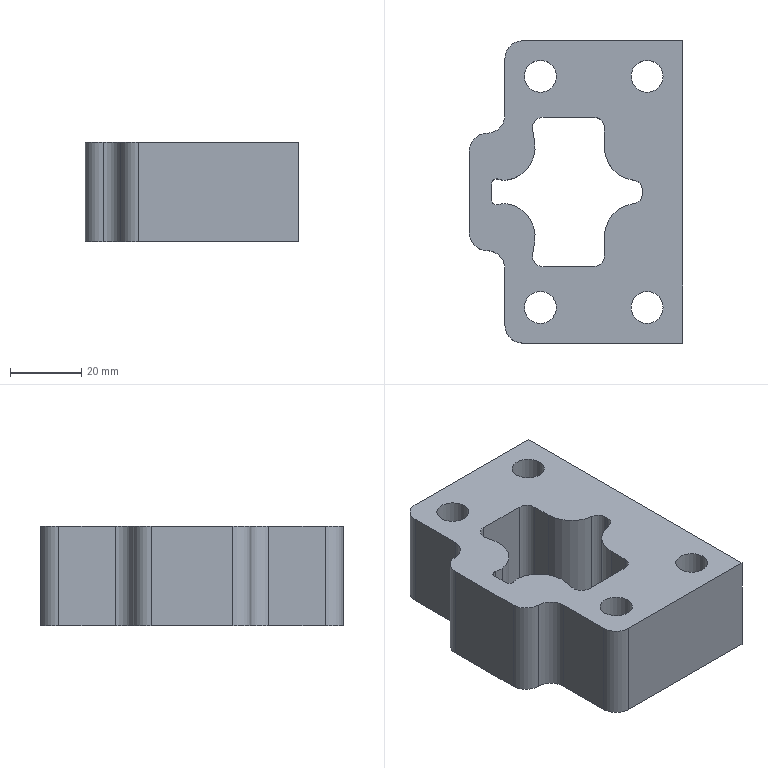Part | STEP file | PN_0024_id1030_x_t | 1 solid | 48 faces | box 60 x 85 x 28 mm | volume 85179 mm3 | cylinder 28 | plane 20 | commonest cylinder face diameters 10 x8 6 x6 9 x4 14 x4 18.5 x4 3 x2
STEP:
#1=CARTESIAN_POINT('',(294.75,11.5,95.));
#2=VERTEX_POINT('',#1);
#3=CARTESIAN_POINT('',(294.75,-11.5,95.));
#4=VERTEX_POINT('',#3);
#5=CARTESIAN_POINT('',(294.75,-13.,95.));
#6=DIRECTION('',(0.,-1.,0.));
#7=VECTOR('',#6,1.);
#8=LINE('',#5,#7);
#9=EDGE_CURVE('',#2,#4,#8,.T.);
#10=ORIENTED_EDGE('',*,*,#9,.F.);
#11=CARTESIAN_POINT('',(294.75,11.5,67.));
#12=VERTEX_POINT('',#11);
#13=CARTESIAN_POINT('',(294.75,11.5,95.));
#14=DIRECTION('',(0.,0.,-1.));
#15=VECTOR('',#14,1.);
#16=LINE('',#13,#15);
#17=EDGE_CURVE('',#2,#12,#16,.T.);
#18=ORIENTED_EDGE('',*,*,#17,.T.);
#19=CARTESIAN_POINT('',(294.75,-11.5,67.));
#20=VERTEX_POINT('',#19);
#21=CARTESIAN_POINT('',(294.75,-13.,67.));
#22=DIRECTION('',(0.,-1.,0.));
#23=VECTOR('',#22,1.);
#24=LINE('',#21,#23);
#25=EDGE_CURVE('',#12,#20,#24,.T.);
#26=ORIENTED_EDGE('',*,*,#25,.T.);
#27=CARTESIAN_POINT('',(294.75,-11.5,95.));
#28=DIRECTION('',(0.,0.,1.));
#29=VECTOR('',#28,1.);
#30=LINE('',#27,#29);
#31=EDGE_CURVE('',#20,#4,#30,.T.);
#32=ORIENTED_EDGE('',*,*,#31,.T.);
#33=EDGE_LOOP('',(#10,#18,#26,#32));
#34=FACE_OUTER_BOUND('',#33,.T.);
#35=CARTESIAN_POINT('',(294.75,-13.,95.));
#36=DIRECTION('',(1.,0.,0.));
#37=DIRECTION('',(0.,-1.,0.));
#38=AXIS2_PLACEMENT_3D('',#35,#36,#37);
#39=PLANE('',#38);
#40=ADVANCED_FACE('',(#34),#39,.F.);
#41=CARTESIAN_POINT('',(354.75,-42.5,95.));
#42=VERTEX_POINT('',#41);
#43=CARTESIAN_POINT('',(309.75,-42.5,95.));
#44=VERTEX_POINT('',#43);
#45=CARTESIAN_POINT('',(265.5,-42.5,95.));
#46=DIRECTION('',(-1.,0.,0.));
#47=VECTOR('',#46,1.);
#48=LINE('',#45,#47);
#49=EDGE_CURVE('',#42,#44,#48,.T.);
#50=ORIENTED_EDGE('',*,*,#49,.T.);
#51=CARTESIAN_POINT('',(309.75,-42.5,67.));
#52=VERTEX_POINT('',#51);
#53=CARTESIAN_POINT('',(309.75,-42.5,67.));
#54=DIRECTION('',(0.,0.,-1.));
#55=VECTOR('',#54,1.);
#56=LINE('',#53,#55);
#57=EDGE_CURVE('',#44,#52,#56,.T.);
#58=ORIENTED_EDGE('',*,*,#57,.T.);
#59=CARTESIAN_POINT('',(354.75,-42.5,67.));
#60=VERTEX_POINT('',#59);
#61=CARTESIAN_POINT('',(265.5,-42.5,67.));
#62=DIRECTION('',(-1.,0.,0.));
#63=VECTOR('',#62,1.);
#64=LINE('',#61,#63);
#65=EDGE_CURVE('',#60,#52,#64,.T.);
#66=ORIENTED_EDGE('',*,*,#65,.F.);
#67=CARTESIAN_POINT('',(354.75,-42.5,95.));
#68=DIRECTION('',(0.,0.,-1.));
#69=VECTOR('',#68,1.);
#70=LINE('',#67,#69);
#71=EDGE_CURVE('',#42,#60,#70,.T.);
#72=ORIENTED_EDGE('',*,*,#71,.F.);
#73=EDGE_LOOP('',(#50,#58,#66,#72));
#74=FACE_OUTER_BOUND('',#73,.T.);
#75=CARTESIAN_POINT('',(265.5,-42.5,95.));
#76=DIRECTION('',(0.,-1.,0.));
#77=DIRECTION('',(-1.,0.,0.));
#78=AXIS2_PLACEMENT_3D('',#75,#76,#77);
#79=PLANE('',#78);
#80=ADVANCED_FACE('',(#74),#79,.T.);
#81=CARTESIAN_POINT('',(354.75,42.5,95.));
#82=VERTEX_POINT('',#81);
#83=CARTESIAN_POINT('',(354.75,3.,95.));
#84=DIRECTION('',(0.,-1.,0.));
#85=VECTOR('',#84,1.);
#86=LINE('',#83,#85);
#87=EDGE_CURVE('',#82,#42,#86,.T.);
#88=ORIENTED_EDGE('',*,*,#87,.T.);
#89=ORIENTED_EDGE('',*,*,#71,.T.);
#90=CARTESIAN_POINT('',(354.75,42.5,67.));
#91=VERTEX_POINT('',#90);
#92=CARTESIAN_POINT('',(354.75,3.,67.));
#93=DIRECTION('',(0.,-1.,0.));
#94=VECTOR('',#93,1.);
#95=LINE('',#92,#94);
#96=EDGE_CURVE('',#91,#60,#95,.T.);
#97=ORIENTED_EDGE('',*,*,#96,.F.);
#98=CARTESIAN_POINT('',(354.75,42.5,95.));
#99=DIRECTION('',(0.,0.,-1.));
#100=VECTOR('',#99,1.);
#101=LINE('',#98,#100);
#102=EDGE_CURVE('',#82,#91,#101,.T.);
#103=ORIENTED_EDGE('',*,*,#102,.F.);
#104=EDGE_LOOP('',(#88,#89,#97,#103));
#105=FACE_OUTER_BOUND('',#104,.T.);
#106=CARTESIAN_POINT('',(354.75,3.,95.));
#107=DIRECTION('',(-1.,0.,0.));
#108=DIRECTION('',(0.,1.,0.));
#109=AXIS2_PLACEMENT_3D('',#106,#107,#108);
#110=PLANE('',#109);
#111=ADVANCED_FACE('',(#105),#110,.F.);
#112=CARTESIAN_POINT('',(310.25,-32.5,95.));
#113=VERTEX_POINT('',#112);
#114=CARTESIAN_POINT('',(314.75,-32.5,95.));
#115=DIRECTION('',(0.,0.,-1.));
#116=DIRECTION('',(-1.,0.,0.));
#117=AXIS2_PLACEMENT_3D('',#114,#115,#116);
#118=CIRCLE('',#117,4.5);
#119=EDGE_CURVE('',#113,#113,#118,.T.);
#120=ORIENTED_EDGE('',*,*,#119,.T.);
#121=EDGE_LOOP('',(#120));
#122=FACE_BOUND('',#121,.T.);
#123=CARTESIAN_POINT('',(340.25,-32.5,95.));
#124=VERTEX_POINT('',#123);
#125=CARTESIAN_POINT('',(344.75,-32.5,95.));
#126=DIRECTION('',(0.,0.,-1.));
#127=DIRECTION('',(-1.,0.,0.));
#128=AXIS2_PLACEMENT_3D('',#125,#126,#127);
#129=CIRCLE('',#128,4.5);
#130=EDGE_CURVE('',#124,#124,#129,.T.);
#131=ORIENTED_EDGE('',*,*,#130,.T.);
#132=EDGE_LOOP('',(#131));
#133=FACE_BOUND('',#132,.T.);
#134=CARTESIAN_POINT('',(310.25,32.5,95.));
#135=VERTEX_POINT('',#134);
#136=CARTESIAN_POINT('',(314.75,32.5,95.));
#137=DIRECTION('',(0.,0.,-1.));
#138=DIRECTION('',(-1.,0.,0.));
#139=AXIS2_PLACEMENT_3D('',#136,#137,#138);
#140=CIRCLE('',#139,4.5);
#141=EDGE_CURVE('',#135,#135,#140,.T.);
#142=ORIENTED_EDGE('',*,*,#141,.T.);
#143=EDGE_LOOP('',(#142));
#144=FACE_BOUND('',#143,.T.);
#145=CARTESIAN_POINT('',(340.25,32.5,95.));
#146=VERTEX_POINT('',#145);
#147=CARTESIAN_POINT('',(344.75,32.5,95.));
#148=DIRECTION('',(0.,0.,-1.));
#149=DIRECTION('',(-1.,0.,0.));
#150=AXIS2_PLACEMENT_3D('',#147,#148,#149);
#151=CIRCLE('',#150,4.5);
#152=EDGE_CURVE('',#146,#146,#151,.T.);
#153=ORIENTED_EDGE('',*,*,#152,.T.);
#154=EDGE_LOOP('',(#153));
#155=FACE_BOUND('',#154,.T.);
#156=CARTESIAN_POINT('',(301.,-2.158,95.));
#157=VERTEX_POINT('',#156);
#158=CARTESIAN_POINT('',(301.,2.158,95.));
#159=VERTEX_POINT('',#158);
#160=CARTESIAN_POINT('',(301.,24.687,95.));
#161=DIRECTION('',(0.,1.,0.));
#162=VECTOR('',#161,1.);
#163=LINE('',#160,#162);
#164=EDGE_CURVE('',#157,#159,#163,.T.);
#165=ORIENTED_EDGE('',*,*,#164,.T.);
#166=CARTESIAN_POINT('',(302.993,3.575,95.));
#167=VERTEX_POINT('',#166);
#168=CARTESIAN_POINT('',(302.5,2.158,95.));
#169=DIRECTION('',(0.,0.,-1.));
#170=DIRECTION('',(-1.,0.,0.));
#171=AXIS2_PLACEMENT_3D('',#168,#169,#170);
#172=CIRCLE('',#171,1.5);
#173=EDGE_CURVE('',#159,#167,#172,.T.);
#174=ORIENTED_EDGE('',*,*,#173,.T.);
#175=CARTESIAN_POINT('',(305.382,3.354,95.));
#176=VERTEX_POINT('',#175);
#177=CARTESIAN_POINT('',(304.635,8.298,95.));
#178=DIRECTION('',(0.,0.,1.));
#179=DIRECTION('',(-1.,0.,0.));
#180=AXIS2_PLACEMENT_3D('',#177,#178,#179);
#181=CIRCLE('',#180,5.);
#182=EDGE_CURVE('',#167,#176,#181,.T.);
#183=ORIENTED_EDGE('',*,*,#182,.T.);
#184=CARTESIAN_POINT('',(313.111,14.097,95.));
#185=VERTEX_POINT('',#184);
#186=CARTESIAN_POINT('',(304.,12.5,95.));
#187=DIRECTION('',(0.,0.,1.));
#188=DIRECTION('',(-1.,0.,0.));
#189=AXIS2_PLACEMENT_3D('',#186,#187,#188);
#190=CIRCLE('',#189,9.25);
#191=EDGE_CURVE('',#176,#185,#190,.T.);
#192=ORIENTED_EDGE('',*,*,#191,.T.);
#193=CARTESIAN_POINT('',(312.518,17.482,95.));
#194=VERTEX_POINT('',#193);
#195=CARTESIAN_POINT('',(298.545,97.182,95.));
#196=DIRECTION('',(-0.1727,0.985,0.));
#197=VECTOR('',#196,1.);
#198=LINE('',#195,#197);
#199=EDGE_CURVE('',#185,#194,#198,.T.);
#200=ORIENTED_EDGE('',*,*,#199,.T.);
#201=CARTESIAN_POINT('',(315.473,21.,95.));
#202=VERTEX_POINT('',#201);
#203=CARTESIAN_POINT('',(315.473,18.,95.));
#204=DIRECTION('',(0.,0.,1.));
#205=DIRECTION('',(-1.,0.,0.));
#206=AXIS2_PLACEMENT_3D('',#203,#204,#205);
#207=CIRCLE('',#206,3.);
#208=EDGE_CURVE('',#202,#194,#207,.T.);
#209=ORIENTED_EDGE('',*,*,#208,.F.);
#210=CARTESIAN_POINT('',(329.75,21.,95.));
#211=VERTEX_POINT('',#210);
#212=CARTESIAN_POINT('',(-114.973,21.,95.));
#213=DIRECTION('',(1.,0.,0.));
#214=VECTOR('',#213,1.);
#215=LINE('',#212,#214);
#216=EDGE_CURVE('',#202,#211,#215,.T.);
#217=ORIENTED_EDGE('',*,*,#216,.T.);
#218=CARTESIAN_POINT('',(332.75,18.,95.));
#219=VERTEX_POINT('',#218);
#220=CARTESIAN_POINT('',(329.75,18.,95.));
#221=DIRECTION('',(0.,0.,1.));
#222=DIRECTION('',(-1.,0.,0.));
#223=AXIS2_PLACEMENT_3D('',#220,#221,#222);
#224=CIRCLE('',#223,3.);
#225=EDGE_CURVE('',#219,#211,#224,.T.);
#226=ORIENTED_EDGE('',*,*,#225,.F.);
#227=CARTESIAN_POINT('',(332.75,12.5,95.));
#228=VERTEX_POINT('',#227);
#229=CARTESIAN_POINT('',(332.75,24.687,95.));
#230=DIRECTION('',(0.,-1.,0.));
#231=VECTOR('',#230,1.);
#232=LINE('',#229,#231);
#233=EDGE_CURVE('',#219,#228,#232,.T.);
#234=ORIENTED_EDGE('',*,*,#233,.T.);
#235=CARTESIAN_POINT('',(340.867,3.32,95.));
#236=VERTEX_POINT('',#235);
#237=CARTESIAN_POINT('',(342.,12.5,95.));
#238=DIRECTION('',(0.,0.,1.));
#239=DIRECTION('',(-1.,0.,0.));
#240=AXIS2_PLACEMENT_3D('',#237,#238,#239);
#241=CIRCLE('',#240,9.25);
#242=EDGE_CURVE('',#228,#236,#241,.T.);
#243=ORIENTED_EDGE('',*,*,#242,.T.);
#244=CARTESIAN_POINT('',(343.5,0.3422,95.));
#245=VERTEX_POINT('',#244);
#246=CARTESIAN_POINT('',(340.5,0.3422,95.));
#247=DIRECTION('',(0.,0.,-1.));
#248=DIRECTION('',(-1.,0.,0.));
#249=AXIS2_PLACEMENT_3D('',#246,#247,#248);
#250=CIRCLE('',#249,3.);
#251=EDGE_CURVE('',#236,#245,#250,.T.);
#252=ORIENTED_EDGE('',*,*,#251,.T.);
#253=CARTESIAN_POINT('',(343.5,-0.3422,95.));
#254=VERTEX_POINT('',#253);
#255=CARTESIAN_POINT('',(343.5,24.687,95.));
#256=DIRECTION('',(0.,-1.,0.));
#257=VECTOR('',#256,1.);
#258=LINE('',#255,#257);
#259=EDGE_CURVE('',#245,#254,#258,.T.);
#260=ORIENTED_EDGE('',*,*,#259,.T.);
#261=CARTESIAN_POINT('',(340.867,-3.32,95.));
#262=VERTEX_POINT('',#261);
#263=CARTESIAN_POINT('',(340.5,-0.3422,95.));
#264=DIRECTION('',(0.,0.,-1.));
#265=DIRECTION('',(-1.,0.,0.));
#266=AXIS2_PLACEMENT_3D('',#263,#264,#265);
#267=CIRCLE('',#266,3.);
#268=EDGE_CURVE('',#254,#262,#267,.T.);
#269=ORIENTED_EDGE('',*,*,#268,.T.);
#270=CARTESIAN_POINT('',(332.75,-12.5,95.));
#271=VERTEX_POINT('',#270);
#272=CARTESIAN_POINT('',(342.,-12.5,95.));
#273=DIRECTION('',(0.,0.,1.));
#274=DIRECTION('',(-1.,0.,0.));
#275=AXIS2_PLACEMENT_3D('',#272,#273,#274);
#276=CIRCLE('',#275,9.25);
#277=EDGE_CURVE('',#262,#271,#276,.T.);
#278=ORIENTED_EDGE('',*,*,#277,.T.);
#279=CARTESIAN_POINT('',(332.75,-18.,95.));
#280=VERTEX_POINT('',#279);
#281=CARTESIAN_POINT('',(332.75,24.687,95.));
#282=DIRECTION('',(0.,-1.,0.));
#283=VECTOR('',#282,1.);
#284=LINE('',#281,#283);
#285=EDGE_CURVE('',#271,#280,#284,.T.);
#286=ORIENTED_EDGE('',*,*,#285,.T.);
#287=CARTESIAN_POINT('',(329.75,-21.,95.));
#288=VERTEX_POINT('',#287);
#289=CARTESIAN_POINT('',(329.75,-18.,95.));
#290=DIRECTION('',(0.,0.,1.));
#291=DIRECTION('',(-1.,0.,0.));
#292=AXIS2_PLACEMENT_3D('',#289,#290,#291);
#293=CIRCLE('',#292,3.);
#294=EDGE_CURVE('',#288,#280,#293,.T.);
#295=ORIENTED_EDGE('',*,*,#294,.F.);
#296=CARTESIAN_POINT('',(315.473,-21.,95.));
#297=VERTEX_POINT('',#296);
#298=CARTESIAN_POINT('',(-114.973,-21.,95.));
#299=DIRECTION('',(-1.,0.,0.));
#300=VECTOR('',#299,1.);
#301=LINE('',#298,#300);
#302=EDGE_CURVE('',#288,#297,#301,.T.);
#303=ORIENTED_EDGE('',*,*,#302,.T.);
#304=CARTESIAN_POINT('',(312.518,-17.482,95.));
#305=VERTEX_POINT('',#304);
#306=CARTESIAN_POINT('',(315.473,-18.,95.));
#307=DIRECTION('',(0.,0.,1.));
#308=DIRECTION('',(-1.,0.,0.));
#309=AXIS2_PLACEMENT_3D('',#306,#307,#308);
#310=CIRCLE('',#309,3.);
#311=EDGE_CURVE('',#305,#297,#310,.T.);
#312=ORIENTED_EDGE('',*,*,#311,.F.);
#313=CARTESIAN_POINT('',(313.111,-14.097,95.));
#314=VERTEX_POINT('',#313);
#315=CARTESIAN_POINT('',(306.943,-49.28,95.));
#316=DIRECTION('',(0.1727,0.985,0.));
#317=VECTOR('',#316,1.);
#318=LINE('',#315,#317);
#319=EDGE_CURVE('',#305,#314,#318,.T.);
#320=ORIENTED_EDGE('',*,*,#319,.T.);
#321=CARTESIAN_POINT('',(305.382,-3.354,95.));
#322=VERTEX_POINT('',#321);
#323=CARTESIAN_POINT('',(304.,-12.5,95.));
#324=DIRECTION('',(0.,0.,1.));
#325=DIRECTION('',(-1.,0.,0.));
#326=AXIS2_PLACEMENT_3D('',#323,#324,#325);
#327=CIRCLE('',#326,9.25);
#328=EDGE_CURVE('',#314,#322,#327,.T.);
#329=ORIENTED_EDGE('',*,*,#328,.T.);
#330=CARTESIAN_POINT('',(302.993,-3.575,95.));
#331=VERTEX_POINT('',#330);
#332=CARTESIAN_POINT('',(304.635,-8.298,95.));
#333=DIRECTION('',(0.,0.,1.));
#334=DIRECTION('',(-1.,0.,0.));
#335=AXIS2_PLACEMENT_3D('',#332,#333,#334);
#336=CIRCLE('',#335,5.);
#337=EDGE_CURVE('',#322,#331,#336,.T.);
#338=ORIENTED_EDGE('',*,*,#337,.T.);
#339=CARTESIAN_POINT('',(302.5,-2.158,95.));
#340=DIRECTION('',(0.,0.,-1.));
#341=DIRECTION('',(-1.,0.,0.));
#342=AXIS2_PLACEMENT_3D('',#339,#340,#341);
#343=CIRCLE('',#342,1.5);
#344=EDGE_CURVE('',#331,#157,#343,.T.);
#345=ORIENTED_EDGE('',*,*,#344,.T.);
#346=EDGE_LOOP('',(#165,#174,#183,#192,#200,#209,#217,#226,#234,#243,#252,#260,#269,#278,#286,#295,#303,#312,#320,#329,#338,#345));
#347=FACE_BOUND('',#346,.T.);
#348=CARTESIAN_POINT('',(309.75,42.5,95.));
#349=VERTEX_POINT('',#348);
#350=CARTESIAN_POINT('',(265.5,42.5,95.));
#351=DIRECTION('',(-1.,0.,0.));
#352=VECTOR('',#351,1.);
#353=LINE('',#350,#352);
#354=EDGE_CURVE('',#82,#349,#353,.T.);
#355=ORIENTED_EDGE('',*,*,#354,.T.);
#356=CARTESIAN_POINT('',(304.75,37.5,95.));
#357=VERTEX_POINT('',#356);
#358=CARTESIAN_POINT('',(309.75,37.5,95.));
#359=DIRECTION('',(0.,0.,1.));
#360=DIRECTION('',(-1.,0.,0.));
#361=AXIS2_PLACEMENT_3D('',#358,#359,#360);
#362=CIRCLE('',#361,5.);
#363=EDGE_CURVE('',#349,#357,#362,.T.);
#364=ORIENTED_EDGE('',*,*,#363,.T.);
#365=CARTESIAN_POINT('',(304.75,21.5,95.));
#366=VERTEX_POINT('',#365);
#367=CARTESIAN_POINT('',(304.75,3.,95.));
#368=DIRECTION('',(0.,-1.,0.));
#369=VECTOR('',#368,1.);
#370=LINE('',#367,#369);
#371=EDGE_CURVE('',#357,#366,#370,.T.);
#372=ORIENTED_EDGE('',*,*,#371,.T.);
#373=CARTESIAN_POINT('',(299.75,16.5,95.));
#374=VERTEX_POINT('',#373);
#375=CARTESIAN_POINT('',(299.75,21.5,95.));
#376=DIRECTION('',(0.,0.,-1.));
#377=DIRECTION('',(-1.,0.,0.));
#378=AXIS2_PLACEMENT_3D('',#375,#376,#377);
#379=CIRCLE('',#378,5.);
#380=EDGE_CURVE('',#366,#374,#379,.T.);
#381=ORIENTED_EDGE('',*,*,#380,.T.);
#382=CARTESIAN_POINT('',(299.75,11.5,95.));
#383=DIRECTION('',(0.,0.,1.));
#384=DIRECTION('',(-1.,0.,0.));
#385=AXIS2_PLACEMENT_3D('',#382,#383,#384);
#386=CIRCLE('',#385,5.);
#387=EDGE_CURVE('',#374,#2,#386,.T.);
#388=ORIENTED_EDGE('',*,*,#387,.T.);
#389=ORIENTED_EDGE('',*,*,#9,.T.);
#390=CARTESIAN_POINT('',(299.75,-16.5,95.));
#391=VERTEX_POINT('',#390);
#392=CARTESIAN_POINT('',(299.75,-11.5,95.));
#393=DIRECTION('',(0.,0.,1.));
#394=DIRECTION('',(-1.,0.,0.));
#395=AXIS2_PLACEMENT_3D('',#392,#393,#394);
#396=CIRCLE('',#395,5.);
#397=EDGE_CURVE('',#4,#391,#396,.T.);
#398=ORIENTED_EDGE('',*,*,#397,.T.);
#399=CARTESIAN_POINT('',(304.75,-21.5,95.));
#400=VERTEX_POINT('',#399);
#401=CARTESIAN_POINT('',(299.75,-21.5,95.));
#402=DIRECTION('',(0.,0.,-1.));
#403=DIRECTION('',(-1.,0.,0.));
#404=AXIS2_PLACEMENT_3D('',#401,#402,#403);
#405=CIRCLE('',#404,5.);
#406=EDGE_CURVE('',#391,#400,#405,.T.);
#407=ORIENTED_EDGE('',*,*,#406,.T.);
#408=CARTESIAN_POINT('',(304.75,-37.5,95.));
#409=VERTEX_POINT('',#408);
#410=CARTESIAN_POINT('',(304.75,3.,95.));
#411=DIRECTION('',(0.,-1.,0.));
#412=VECTOR('',#411,1.);
#413=LINE('',#410,#412);
#414=EDGE_CURVE('',#400,#409,#413,.T.);
#415=ORIENTED_EDGE('',*,*,#414,.T.);
#416=CARTESIAN_POINT('',(309.75,-37.5,95.));
#417=DIRECTION('',(0.,0.,1.));
#418=DIRECTION('',(-1.,0.,0.));
#419=AXIS2_PLACEMENT_3D('',#416,#417,#418);
#420=CIRCLE('',#419,5.);
#421=EDGE_CURVE('',#409,#44,#420,.T.);
#422=ORIENTED_EDGE('',*,*,#421,.T.);
#423=ORIENTED_EDGE('',*,*,#49,.F.);
#424=ORIENTED_EDGE('',*,*,#87,.F.);
#425=EDGE_LOOP('',(#355,#364,#372,#381,#388,#389,#398,#407,#415,#422,#423,#424));
#426=FACE_BOUND('',#425,.T.);
#427=CARTESIAN_POINT('',(265.5,3.,95.));
#428=DIRECTION('',(0.,0.,-1.));
#429=DIRECTION('',(-1.,0.,0.));
#430=AXIS2_PLACEMENT_3D('',#427,#428,#429);
#431=PLANE('',#430);
#432=ADVANCED_FACE('',(#122,#133,#144,#155,#347,#426),#431,.F.);
#433=CARTESIAN_POINT('',(321.75,-32.5,67.));
#434=VERTEX_POINT('',#433);
#435=CARTESIAN_POINT('',(314.75,-32.5,67.));
#436=DIRECTION('',(0.,0.,1.));
#437=DIRECTION('',(1.,0.,0.));
#438=AXIS2_PLACEMENT_3D('',#435,#436,#437);
#439=CIRCLE('',#438,7.);
#440=EDGE_CURVE('',#434,#434,#439,.T.);
#441=ORIENTED_EDGE('',*,*,#440,.T.);
#442=EDGE_LOOP('',(#441));
#443=FACE_BOUND('',#442,.T.);
#444=CARTESIAN_POINT('',(337.75,-32.5,67.));
#445=VERTEX_POINT('',#444);
#446=CARTESIAN_POINT('',(344.75,-32.5,67.));
#447=DIRECTION('',(0.,0.,-1.));
#448=DIRECTION('',(-1.,0.,0.));
#449=AXIS2_PLACEMENT_3D('',#446,#447,#448);
#450=CIRCLE('',#449,7.);
#451=EDGE_CURVE('',#445,#445,#450,.T.);
#452=ORIENTED_EDGE('',*,*,#451,.F.);
#453=EDGE_LOOP('',(#452));
#454=FACE_BOUND('',#453,.T.);
#455=CARTESIAN_POINT('',(321.75,32.5,67.));
#456=VERTEX_POINT('',#455);
#457=CARTESIAN_POINT('',(314.75,32.5,67.));
#458=DIRECTION('',(0.,0.,-1.));
#459=DIRECTION('',(1.,0.,0.));
#460=AXIS2_PLACEMENT_3D('',#457,#458,#459);
#461=CIRCLE('',#460,7.);
#462=EDGE_CURVE('',#456,#456,#461,.T.);
#463=ORIENTED_EDGE('',*,*,#462,.F.);
#464=EDGE_LOOP('',(#463));
#465=FACE_BOUND('',#464,.T.);
#466=CARTESIAN_POINT('',(337.75,32.5,67.));
#467=VERTEX_POINT('',#466);
#468=CARTESIAN_POINT('',(344.75,32.5,67.));
#469=DIRECTION('',(0.,0.,1.));
#470=DIRECTION('',(-1.,0.,0.));
#471=AXIS2_PLACEMENT_3D('',#468,#469,#470);
#472=CIRCLE('',#471,7.);
#473=EDGE_CURVE('',#467,#467,#472,.T.);
#474=ORIENTED_EDGE('',*,*,#473,.T.);
#475=EDGE_LOOP('',(#474));
#476=FACE_BOUND('',#475,.T.);
#477=CARTESIAN_POINT('',(343.5,-0.3422,67.));
#478=VERTEX_POINT('',#477);
#479=CARTESIAN_POINT('',(340.867,-3.32,67.));
#480=VERTEX_POINT('',#479);
#481=CARTESIAN_POINT('',(340.5,-0.3422,67.));
#482=DIRECTION('',(0.,0.,-1.));
#483=DIRECTION('',(-1.,0.,0.));
#484=AXIS2_PLACEMENT_3D('',#481,#482,#483);
#485=CIRCLE('',#484,3.);
#486=EDGE_CURVE('',#478,#480,#485,.T.);
#487=ORIENTED_EDGE('',*,*,#486,.F.);
#488=CARTESIAN_POINT('',(343.5,0.3422,67.));
#489=VERTEX_POINT('',#488);
#490=CARTESIAN_POINT('',(343.5,3.,67.));
#491=DIRECTION('',(0.,-1.,0.));
#492=VECTOR('',#491,1.);
#493=LINE('',#490,#492);
#494=EDGE_CURVE('',#489,#478,#493,.T.);
#495=ORIENTED_EDGE('',*,*,#494,.F.);
#496=CARTESIAN_POINT('',(340.867,3.32,67.));
#497=VERTEX_POINT('',#496);
#498=CARTESIAN_POINT('',(340.5,0.3422,67.));
#499=DIRECTION('',(0.,0.,-1.));
#500=DIRECTION('',(-1.,0.,0.));
#501=AXIS2_PLACEMENT_3D('',#498,#499,#500);
#502=CIRCLE('',#501,3.);
#503=EDGE_CURVE('',#497,#489,#502,.T.);
#504=ORIENTED_EDGE('',*,*,#503,.F.);
#505=CARTESIAN_POINT('',(332.75,12.5,67.));
#506=VERTEX_POINT('',#505);
#507=CARTESIAN_POINT('',(342.,12.5,67.));
#508=DIRECTION('',(0.,0.,1.));
#509=DIRECTION('',(-1.,0.,0.));
#510=AXIS2_PLACEMENT_3D('',#507,#508,#509);
#511=CIRCLE('',#510,9.25);
#512=EDGE_CURVE('',#506,#497,#511,.T.);
#513=ORIENTED_EDGE('',*,*,#512,.F.);
#514=CARTESIAN_POINT('',(332.75,18.,67.));
#515=VERTEX_POINT('',#514);
#516=CARTESIAN_POINT('',(332.75,3.,67.));
#517=DIRECTION('',(0.,-1.,0.));
#518=VECTOR('',#517,1.);
#519=LINE('',#516,#518);
#520=EDGE_CURVE('',#515,#506,#519,.T.);
#521=ORIENTED_EDGE('',*,*,#520,.F.);
#522=CARTESIAN_POINT('',(329.75,21.,67.));
#523=VERTEX_POINT('',#522);
#524=CARTESIAN_POINT('',(329.75,18.,67.));
#525=DIRECTION('',(0.,0.,-1.));
#526=DIRECTION('',(-1.,0.,0.));
#527=AXIS2_PLACEMENT_3D('',#524,#525,#526);
#528=CIRCLE('',#527,3.);
#529=EDGE_CURVE('',#523,#515,#528,.T.);
#530=ORIENTED_EDGE('',*,*,#529,.F.);
#531=CARTESIAN_POINT('',(315.473,21.,67.));
#532=VERTEX_POINT('',#531);
#533=CARTESIAN_POINT('',(265.5,21.,67.));
#534=DIRECTION('',(1.,0.,0.));
#535=VECTOR('',#534,1.);
#536=LINE('',#533,#535);
#537=EDGE_CURVE('',#532,#523,#536,.T.);
#538=ORIENTED_EDGE('',*,*,#537,.F.);
#539=CARTESIAN_POINT('',(312.518,17.482,67.));
#540=VERTEX_POINT('',#539);
#541=CARTESIAN_POINT('',(315.473,18.,67.));
#542=DIRECTION('',(0.,0.,-1.));
#543=DIRECTION('',(-1.,0.,0.));
#544=AXIS2_PLACEMENT_3D('',#541,#542,#543);
#545=CIRCLE('',#544,3.);
#546=EDGE_CURVE('',#540,#532,#545,.T.);
#547=ORIENTED_EDGE('',*,*,#546,.F.);
#548=CARTESIAN_POINT('',(313.111,14.097,67.));
#549=VERTEX_POINT('',#548);
#550=CARTESIAN_POINT('',(313.579,11.429,67.));
#551=DIRECTION('',(-0.1727,0.985,0.));
#552=VECTOR('',#551,1.);
#553=LINE('',#550,#552);
#554=EDGE_CURVE('',#549,#540,#553,.T.);
#555=ORIENTED_EDGE('',*,*,#554,.F.);
#556=CARTESIAN_POINT('',(305.382,3.354,67.));
#557=VERTEX_POINT('',#556);
#558=CARTESIAN_POINT('',(304.,12.5,67.));
#559=DIRECTION('',(0.,0.,1.));
#560=DIRECTION('',(-1.,0.,0.));
#561=AXIS2_PLACEMENT_3D('',#558,#559,#560);
#562=CIRCLE('',#561,9.25);
#563=EDGE_CURVE('',#557,#549,#562,.T.);
#564=ORIENTED_EDGE('',*,*,#563,.F.);
#565=CARTESIAN_POINT('',(302.993,3.575,67.));
#566=VERTEX_POINT('',#565);
#567=CARTESIAN_POINT('',(304.635,8.298,67.));
#568=DIRECTION('',(0.,0.,1.));
#569=DIRECTION('',(-1.,0.,0.));
#570=AXIS2_PLACEMENT_3D('',#567,#568,#569);
#571=CIRCLE('',#570,5.);
#572=EDGE_CURVE('',#566,#557,#571,.T.);
#573=ORIENTED_EDGE('',*,*,#572,.F.);
#574=CARTESIAN_POINT('',(301.,2.158,67.));
#575=VERTEX_POINT('',#574);
#576=CARTESIAN_POINT('',(302.5,2.158,67.));
#577=DIRECTION('',(0.,0.,-1.));
#578=DIRECTION('',(-1.,0.,0.));
#579=AXIS2_PLACEMENT_3D('',#576,#577,#578);
#580=CIRCLE('',#579,1.5);
#581=EDGE_CURVE('',#575,#566,#580,.T.);
#582=ORIENTED_EDGE('',*,*,#581,.F.);
#583=CARTESIAN_POINT('',(301.,-2.158,67.));
#584=VERTEX_POINT('',#583);
#585=CARTESIAN_POINT('',(301.,3.,67.));
#586=DIRECTION('',(0.,1.,0.));
#587=VECTOR('',#586,1.);
#588=LINE('',#585,#587);
#589=EDGE_CURVE('',#584,#575,#588,.T.);
#590=ORIENTED_EDGE('',*,*,#589,.F.);
#591=CARTESIAN_POINT('',(302.993,-3.575,67.));
#592=VERTEX_POINT('',#591);
#593=CARTESIAN_POINT('',(302.5,-2.158,67.));
#594=DIRECTION('',(0.,0.,-1.));
#595=DIRECTION('',(-1.,0.,0.));
#596=AXIS2_PLACEMENT_3D('',#593,#594,#595);
#597=CIRCLE('',#596,1.5);
#598=EDGE_CURVE('',#592,#584,#597,.T.);
#599=ORIENTED_EDGE('',*,*,#598,.F.);
#600=CARTESIAN_POINT('',(305.382,-3.354,67.));
#601=VERTEX_POINT('',#600);
#602=CARTESIAN_POINT('',(304.635,-8.298,67.));
#603=DIRECTION('',(0.,0.,1.));
#604=DIRECTION('',(-1.,0.,0.));
#605=AXIS2_PLACEMENT_3D('',#602,#603,#604);
#606=CIRCLE('',#605,5.);
#607=EDGE_CURVE('',#601,#592,#606,.T.);
#608=ORIENTED_EDGE('',*,*,#607,.F.);
#609=CARTESIAN_POINT('',(313.111,-14.097,67.));
#610=VERTEX_POINT('',#609);
#611=CARTESIAN_POINT('',(304.,-12.5,67.));
#612=DIRECTION('',(0.,0.,1.));
#613=DIRECTION('',(-1.,0.,0.));
#614=AXIS2_PLACEMENT_3D('',#611,#612,#613);
#615=CIRCLE('',#614,9.25);
#616=EDGE_CURVE('',#610,#601,#615,.T.);
#617=ORIENTED_EDGE('',*,*,#616,.F.);
#618=CARTESIAN_POINT('',(312.518,-17.482,67.));
#619=VERTEX_POINT('',#618);
#620=CARTESIAN_POINT('',(314.599,-5.608,67.));
#621=DIRECTION('',(0.1727,0.985,0.));
#622=VECTOR('',#621,1.);
#623=LINE('',#620,#622);
#624=EDGE_CURVE('',#619,#610,#623,.T.);
#625=ORIENTED_EDGE('',*,*,#624,.F.);
#626=CARTESIAN_POINT('',(315.473,-21.,67.));
#627=VERTEX_POINT('',#626);
#628=CARTESIAN_POINT('',(315.473,-18.,67.));
#629=DIRECTION('',(0.,0.,-1.));
#630=DIRECTION('',(-1.,0.,0.));
#631=AXIS2_PLACEMENT_3D('',#628,#629,#630);
#632=CIRCLE('',#631,3.);
#633=EDGE_CURVE('',#627,#619,#632,.T.);
#634=ORIENTED_EDGE('',*,*,#633,.F.);
#635=CARTESIAN_POINT('',(329.75,-21.,67.));
#636=VERTEX_POINT('',#635);
#637=CARTESIAN_POINT('',(265.5,-21.,67.));
#638=DIRECTION('',(-1.,0.,0.));
#639=VECTOR('',#638,1.);
#640=LINE('',#637,#639);
#641=EDGE_CURVE('',#636,#627,#640,.T.);
#642=ORIENTED_EDGE('',*,*,#641,.F.);
#643=CARTESIAN_POINT('',(332.75,-18.,67.));
#644=VERTEX_POINT('',#643);
#645=CARTESIAN_POINT('',(329.75,-18.,67.));
#646=DIRECTION('',(0.,0.,-1.));
#647=DIRECTION('',(-1.,0.,0.));
#648=AXIS2_PLACEMENT_3D('',#645,#646,#647);
#649=CIRCLE('',#648,3.);
#650=EDGE_CURVE('',#644,#636,#649,.T.);
#651=ORIENTED_EDGE('',*,*,#650,.F.);
#652=CARTESIAN_POINT('',(332.75,-12.5,67.));
#653=VERTEX_POINT('',#652);
#654=CARTESIAN_POINT('',(332.75,3.,67.));
#655=DIRECTION('',(0.,-1.,0.));
#656=VECTOR('',#655,1.);
#657=LINE('',#654,#656);
#658=EDGE_CURVE('',#653,#644,#657,.T.);
#659=ORIENTED_EDGE('',*,*,#658,.F.);
#660=CARTESIAN_POINT('',(342.,-12.5,67.));
#661=DIRECTION('',(0.,0.,1.));
#662=DIRECTION('',(-1.,0.,0.));
#663=AXIS2_PLACEMENT_3D('',#660,#661,#662);
#664=CIRCLE('',#663,9.25);
#665=EDGE_CURVE('',#480,#653,#664,.T.);
#666=ORIENTED_EDGE('',*,*,#665,.F.);
#667=EDGE_LOOP('',(#487,#495,#504,#513,#521,#530,#538,#547,#555,#564,#573,#582,#590,#599,#608,#617,#625,#634,#642,#651,#659,#666));
#668=FACE_BOUND('',#667,.T.);
#669=CARTESIAN_POINT('',(304.75,37.5,67.));
#670=VERTEX_POINT('',#669);
#671=CARTESIAN_POINT('',(304.75,21.5,67.));
#672=VERTEX_POINT('',#671);
#673=CARTESIAN_POINT('',(304.75,3.,67.));
#674=DIRECTION('',(0.,-1.,0.));
#675=VECTOR('',#674,1.);
#676=LINE('',#673,#675);
#677=EDGE_CURVE('',#670,#672,#676,.T.);
#678=ORIENTED_EDGE('',*,*,#677,.F.);
#679=CARTESIAN_POINT('',(309.75,42.5,67.));
#680=VERTEX_POINT('',#679);
#681=CARTESIAN_POINT('',(309.75,37.5,67.));
#682=DIRECTION('',(0.,0.,-1.));
#683=DIRECTION('',(-1.,0.,0.));
#684=AXIS2_PLACEMENT_3D('',#681,#682,#683);
#685=CIRCLE('',#684,5.);
#686=EDGE_CURVE('',#670,#680,#685,.T.);
#687=ORIENTED_EDGE('',*,*,#686,.T.);
#688=CARTESIAN_POINT('',(265.5,42.5,67.));
#689=DIRECTION('',(-1.,0.,0.));
#690=VECTOR('',#689,1.);
#691=LINE('',#688,#690);
#692=EDGE_CURVE('',#91,#680,#691,.T.);
#693=ORIENTED_EDGE('',*,*,#692,.F.);
#694=ORIENTED_EDGE('',*,*,#96,.T.);
#695=ORIENTED_EDGE('',*,*,#65,.T.);
#696=CARTESIAN_POINT('',(304.75,-37.5,67.));
#697=VERTEX_POINT('',#696);
#698=CARTESIAN_POINT('',(309.75,-37.5,67.));
#699=DIRECTION('',(0.,0.,-1.));
#700=DIRECTION('',(-1.,0.,0.));
#701=AXIS2_PLACEMENT_3D('',#698,#699,#700);
#702=CIRCLE('',#701,5.);
#703=EDGE_CURVE('',#52,#697,#702,.T.);
#704=ORIENTED_EDGE('',*,*,#703,.T.);
#705=CARTESIAN_POINT('',(304.75,-21.5,67.));
#706=VERTEX_POINT('',#705);
#707=CARTESIAN_POINT('',(304.75,3.,67.));
#708=DIRECTION('',(0.,-1.,0.));
#709=VECTOR('',#708,1.);
#710=LINE('',#707,#709);
#711=EDGE_CURVE('',#706,#697,#710,.T.);
#712=ORIENTED_EDGE('',*,*,#711,.F.);
#713=CARTESIAN_POINT('',(299.75,-16.5,67.));
#714=VERTEX_POINT('',#713);
#715=CARTESIAN_POINT('',(299.75,-21.5,67.));
#716=DIRECTION('',(0.,0.,-1.));
#717=DIRECTION('',(-1.,0.,0.));
#718=AXIS2_PLACEMENT_3D('',#715,#716,#717);
#719=CIRCLE('',#718,5.);
#720=EDGE_CURVE('',#714,#706,#719,.T.);
#721=ORIENTED_EDGE('',*,*,#720,.F.);
#722=CARTESIAN_POINT('',(299.75,-11.5,67.));
#723=DIRECTION('',(0.,0.,-1.));
#724=DIRECTION('',(-1.,0.,0.));
#725=AXIS2_PLACEMENT_3D('',#722,#723,#724);
#726=CIRCLE('',#725,5.);
#727=EDGE_CURVE('',#714,#20,#726,.T.);
#728=ORIENTED_EDGE('',*,*,#727,.T.);
#729=ORIENTED_EDGE('',*,*,#25,.F.);
#730=CARTESIAN_POINT('',(299.75,16.5,67.));
#731=VERTEX_POINT('',#730);
#732=CARTESIAN_POINT('',(299.75,11.5,67.));
#733=DIRECTION('',(0.,0.,-1.));
#734=DIRECTION('',(-1.,0.,0.));
#735=AXIS2_PLACEMENT_3D('',#732,#733,#734);
#736=CIRCLE('',#735,5.);
#737=EDGE_CURVE('',#12,#731,#736,.T.);
#738=ORIENTED_EDGE('',*,*,#737,.T.);
#739=CARTESIAN_POINT('',(299.75,21.5,67.));
#740=DIRECTION('',(0.,0.,1.));
#741=DIRECTION('',(-1.,0.,0.));
#742=AXIS2_PLACEMENT_3D('',#739,#740,#741);
#743=CIRCLE('',#742,5.);
#744=EDGE_CURVE('',#731,#672,#743,.T.);
#745=ORIENTED_EDGE('',*,*,#744,.T.);
#746=EDGE_LOOP('',(#678,#687,#693,#694,#695,#704,#712,#721,#728,#729,#738,#745));
#747=FACE_BOUND('',#746,.T.);
#748=CARTESIAN_POINT('',(265.5,3.,67.));
#749=DIRECTION('',(0.,0.,-1.));
#750=DIRECTION('',(-1.,0.,0.));
#751=AXIS2_PLACEMENT_3D('',#748,#749,#750);
#752=PLANE('',#751);
#753=ADVANCED_FACE('',(#443,#454,#465,#476,#668,#747),#752,.T.);
#754=ORIENTED_EDGE('',*,*,#692,.T.);
#755=CARTESIAN_POINT('',(309.75,42.5,95.));
#756=DIRECTION('',(0.,0.,1.));
#757=VECTOR('',#756,1.);
#758=LINE('',#755,#757);
#759=EDGE_CURVE('',#680,#349,#758,.T.);
#760=ORIENTED_EDGE('',*,*,#759,.T.);
#761=ORIENTED_EDGE('',*,*,#354,.F.);
#762=ORIENTED_EDGE('',*,*,#102,.T.);
#763=EDGE_LOOP('',(#754,#760,#761,#762));
#764=FACE_OUTER_BOUND('',#763,.T.);
#765=CARTESIAN_POINT('',(265.5,42.5,95.));
#766=DIRECTION('',(0.,1.,0.));
#767=DIRECTION('',(1.,0.,0.));
#768=AXIS2_PLACEMENT_3D('',#765,#766,#767);
#769=PLANE('',#768);
#770=ADVANCED_FACE('',(#764),#769,.T.);
#771=ORIENTED_EDGE('',*,*,#371,.F.);
#772=CARTESIAN_POINT('',(304.75,37.5,67.));
#773=DIRECTION('',(0.,0.,-1.));
#774=VECTOR('',#773,1.);
#775=LINE('',#772,#774);
#776=EDGE_CURVE('',#357,#670,#775,.T.);
#777=ORIENTED_EDGE('',*,*,#776,.T.);
#778=ORIENTED_EDGE('',*,*,#677,.T.);
#779=CARTESIAN_POINT('',(304.75,21.5,81.));
#780=DIRECTION('',(0.,0.,1.));
#781=VECTOR('',#780,1.);
#782=LINE('',#779,#781);
#783=EDGE_CURVE('',#672,#366,#782,.T.);
#784=ORIENTED_EDGE('',*,*,#783,.T.);
#785=EDGE_LOOP('',(#771,#777,#778,#784));
#786=FACE_OUTER_BOUND('',#785,.T.);
#787=CARTESIAN_POINT('',(304.75,34.5,81.));
#788=DIRECTION('',(1.,0.,0.));
#789=DIRECTION('',(0.,0.,-1.));
#790=AXIS2_PLACEMENT_3D('',#787,#788,#789);
#791=PLANE('',#790);
#792=ADVANCED_FACE('',(#786),#791,.F.);
#793=ORIENTED_EDGE('',*,*,#380,.F.);
#794=ORIENTED_EDGE('',*,*,#783,.F.);
#795=ORIENTED_EDGE('',*,*,#744,.F.);
#796=CARTESIAN_POINT('',(299.75,16.5,81.));
#797=DIRECTION('',(0.,0.,-1.));
#798=VECTOR('',#797,1.);
#799=LINE('',#796,#798);
#800=EDGE_CURVE('',#374,#731,#799,.T.);
#801=ORIENTED_EDGE('',*,*,#800,.F.);
#802=EDGE_LOOP('',(#793,#794,#795,#801));
#803=FACE_OUTER_BOUND('',#802,.T.);
#804=CARTESIAN_POINT('',(299.75,21.5,81.));
#805=DIRECTION('',(0.,0.,-1.));
#806=DIRECTION('',(-1.,0.,0.));
#807=AXIS2_PLACEMENT_3D('',#804,#805,#806);
#808=CYLINDRICAL_SURFACE('',#807,5.);
#809=ADVANCED_FACE('',(#803),#808,.F.);
#810=CARTESIAN_POINT('',(299.75,-16.5,118.));
#811=DIRECTION('',(0.,0.,1.));
#812=VECTOR('',#811,1.);
#813=LINE('',#810,#812);
#814=EDGE_CURVE('',#714,#391,#813,.T.);
#815=ORIENTED_EDGE('',*,*,#814,.F.);
#816=ORIENTED_EDGE('',*,*,#720,.T.);
#817=CARTESIAN_POINT('',(304.75,-21.5,118.));
#818=DIRECTION('',(0.,0.,1.));
#819=VECTOR('',#818,1.);
#820=LINE('',#817,#819);
#821=EDGE_CURVE('',#706,#400,#820,.T.);
#822=ORIENTED_EDGE('',*,*,#821,.T.);
#823=ORIENTED_EDGE('',*,*,#406,.F.);
#824=EDGE_LOOP('',(#815,#816,#822,#823));
#825=FACE_OUTER_BOUND('',#824,.T.);
#826=CARTESIAN_POINT('',(299.75,-21.5,118.));
#827=DIRECTION('',(0.,0.,-1.));
#828=DIRECTION('',(-1.,0.,0.));
#829=AXIS2_PLACEMENT_3D('',#826,#827,#828);
#830=CYLINDRICAL_SURFACE('',#829,5.);
#831=ADVANCED_FACE('',(#825),#830,.F.);
#832=ORIENTED_EDGE('',*,*,#711,.T.);
#833=CARTESIAN_POINT('',(304.75,-37.5,95.));
#834=DIRECTION('',(0.,0.,1.));
#835=VECTOR('',#834,1.);
#836=LINE('',#833,#835);
#837=EDGE_CURVE('',#697,#409,#836,.T.);
#838=ORIENTED_EDGE('',*,*,#837,.T.);
#839=ORIENTED_EDGE('',*,*,#414,.F.);
#840=ORIENTED_EDGE('',*,*,#821,.F.);
#841=EDGE_LOOP('',(#832,#838,#839,#840));
#842=FACE_OUTER_BOUND('',#841,.T.);
#843=CARTESIAN_POINT('',(304.75,-52.5,118.));
#844=DIRECTION('',(1.,0.,0.));
#845=DIRECTION('',(0.,0.,-1.));
#846=AXIS2_PLACEMENT_3D('',#843,#844,#845);
#847=PLANE('',#846);
#848=ADVANCED_FACE('',(#842),#847,.F.);
#849=ORIENTED_EDGE('',*,*,#486,.T.);
#850=CARTESIAN_POINT('',(340.867,-3.32,11.));
#851=DIRECTION('',(0.,0.,1.));
#852=VECTOR('',#851,1.);
#853=LINE('',#850,#852);
#854=EDGE_CURVE('',#480,#262,#853,.T.);
#855=ORIENTED_EDGE('',*,*,#854,.T.);
#856=ORIENTED_EDGE('',*,*,#268,.F.);
#857=CARTESIAN_POINT('',(343.5,-0.3422,11.));
#858=DIRECTION('',(0.,0.,1.));
#859=VECTOR('',#858,1.);
#860=LINE('',#857,#859);
#861=EDGE_CURVE('',#478,#254,#860,.T.);
#862=ORIENTED_EDGE('',*,*,#861,.F.);
#863=EDGE_LOOP('',(#849,#855,#856,#862));
#864=FACE_OUTER_BOUND('',#863,.T.);
#865=CARTESIAN_POINT('',(340.5,-0.3422,11.));
#866=DIRECTION('',(0.,0.,-1.));
#867=DIRECTION('',(-1.,0.,0.));
#868=AXIS2_PLACEMENT_3D('',#865,#866,#867);
#869=CYLINDRICAL_SURFACE('',#868,3.);
#870=ADVANCED_FACE('',(#864),#869,.F.);
#871=ORIENTED_EDGE('',*,*,#665,.T.);
#872=CARTESIAN_POINT('',(332.75,-12.5,11.));
#873=DIRECTION('',(0.,0.,1.));
#874=VECTOR('',#873,1.);
#875=LINE('',#872,#874);
#876=EDGE_CURVE('',#653,#271,#875,.T.);
#877=ORIENTED_EDGE('',*,*,#876,.T.);
#878=ORIENTED_EDGE('',*,*,#277,.F.);
#879=ORIENTED_EDGE('',*,*,#854,.F.);
#880=EDGE_LOOP('',(#871,#877,#878,#879));
#881=FACE_OUTER_BOUND('',#880,.T.);
#882=CARTESIAN_POINT('',(342.,-12.5,11.));
#883=DIRECTION('',(0.,0.,-1.));
#884=DIRECTION('',(-1.,0.,0.));
#885=AXIS2_PLACEMENT_3D('',#882,#883,#884);
#886=CYLINDRICAL_SURFACE('',#885,9.25);
#887=ADVANCED_FACE('',(#881),#886,.T.);
#888=ORIENTED_EDGE('',*,*,#658,.T.);
#889=CARTESIAN_POINT('',(332.75,-18.,11.));
#890=DIRECTION('',(0.,0.,1.));
#891=VECTOR('',#890,1.);
#892=LINE('',#889,#891);
#893=EDGE_CURVE('',#644,#280,#892,.T.);
#894=ORIENTED_EDGE('',*,*,#893,.T.);
#895=ORIENTED_EDGE('',*,*,#285,.F.);
#896=ORIENTED_EDGE('',*,*,#876,.F.);
#897=EDGE_LOOP('',(#888,#894,#895,#896));
#898=FACE_OUTER_BOUND('',#897,.T.);
#899=CARTESIAN_POINT('',(332.75,-71.15,11.));
#900=DIRECTION('',(-1.,0.,0.));
#901=DIRECTION('',(0.,1.,0.));
#902=AXIS2_PLACEMENT_3D('',#899,#900,#901);
#903=PLANE('',#902);
#904=ADVANCED_FACE('',(#898),#903,.T.);
#905=ORIENTED_EDGE('',*,*,#641,.T.);
#906=CARTESIAN_POINT('',(315.473,-21.,11.));
#907=DIRECTION('',(0.,0.,1.));
#908=VECTOR('',#907,1.);
#909=LINE('',#906,#908);
#910=EDGE_CURVE('',#627,#297,#909,.T.);
#911=ORIENTED_EDGE('',*,*,#910,.T.);
#912=ORIENTED_EDGE('',*,*,#302,.F.);
#913=CARTESIAN_POINT('',(329.75,-21.,11.));
#914=DIRECTION('',(0.,0.,-1.));
#915=VECTOR('',#914,1.);
#916=LINE('',#913,#915);
#917=EDGE_CURVE('',#288,#636,#916,.T.);
#918=ORIENTED_EDGE('',*,*,#917,.T.);
#919=EDGE_LOOP('',(#905,#911,#912,#918));
#920=FACE_OUTER_BOUND('',#919,.T.);
#921=CARTESIAN_POINT('',(546.19,-21.,11.));
#922=DIRECTION('',(0.,-1.,0.));
#923=DIRECTION('',(-1.,0.,0.));
#924=AXIS2_PLACEMENT_3D('',#921,#922,#923);
#925=PLANE('',#924);
#926=ADVANCED_FACE('',(#920),#925,.F.);
#927=ORIENTED_EDGE('',*,*,#624,.T.);
#928=CARTESIAN_POINT('',(313.111,-14.097,11.));
#929=DIRECTION('',(0.,0.,1.));
#930=VECTOR('',#929,1.);
#931=LINE('',#928,#930);
#932=EDGE_CURVE('',#610,#314,#931,.T.);
#933=ORIENTED_EDGE('',*,*,#932,.T.);
#934=ORIENTED_EDGE('',*,*,#319,.F.);
#935=CARTESIAN_POINT('',(312.518,-17.482,11.));
#936=DIRECTION('',(0.,0.,-1.));
#937=VECTOR('',#936,1.);
#938=LINE('',#935,#937);
#939=EDGE_CURVE('',#305,#619,#938,.T.);
#940=ORIENTED_EDGE('',*,*,#939,.T.);
#941=EDGE_LOOP('',(#927,#933,#934,#940));
#942=FACE_OUTER_BOUND('',#941,.T.);
#943=CARTESIAN_POINT('',(313.111,-14.097,11.));
#944=DIRECTION('',(0.985,-0.1727,0.));
#945=DIRECTION('',(-0.1727,-0.985,0.));
#946=AXIS2_PLACEMENT_3D('',#943,#944,#945);
#947=PLANE('',#946);
#948=ADVANCED_FACE('',(#942),#947,.T.);
#949=ORIENTED_EDGE('',*,*,#616,.T.);
#950=CARTESIAN_POINT('',(305.382,-3.354,49.5));
#951=DIRECTION('',(0.,0.,-1.));
#952=VECTOR('',#951,1.);
#953=LINE('',#950,#952);
#954=EDGE_CURVE('',#322,#601,#953,.T.);
#955=ORIENTED_EDGE('',*,*,#954,.F.);
#956=ORIENTED_EDGE('',*,*,#328,.F.);
#957=ORIENTED_EDGE('',*,*,#932,.F.);
#958=EDGE_LOOP('',(#949,#955,#956,#957));
#959=FACE_OUTER_BOUND('',#958,.T.);
#960=CARTESIAN_POINT('',(304.,-12.5,11.));
#961=DIRECTION('',(0.,0.,-1.));
#962=DIRECTION('',(-1.,0.,0.));
#963=AXIS2_PLACEMENT_3D('',#960,#961,#962);
#964=CYLINDRICAL_SURFACE('',#963,9.25);
#965=ADVANCED_FACE('',(#959),#964,.T.);
#966=ORIENTED_EDGE('',*,*,#563,.T.);
#967=CARTESIAN_POINT('',(313.111,14.097,11.));
#968=DIRECTION('',(0.,0.,1.));
#969=VECTOR('',#968,1.);
#970=LINE('',#967,#969);
#971=EDGE_CURVE('',#549,#185,#970,.T.);
#972=ORIENTED_EDGE('',*,*,#971,.T.);
#973=ORIENTED_EDGE('',*,*,#191,.F.);
#974=CARTESIAN_POINT('',(305.382,3.354,49.5));
#975=DIRECTION('',(0.,0.,-1.));
#976=VECTOR('',#975,1.);
#977=LINE('',#974,#976);
#978=EDGE_CURVE('',#176,#557,#977,.T.);
#979=ORIENTED_EDGE('',*,*,#978,.T.);
#980=EDGE_LOOP('',(#966,#972,#973,#979));
#981=FACE_OUTER_BOUND('',#980,.T.);
#982=CARTESIAN_POINT('',(304.,12.5,11.));
#983=DIRECTION('',(0.,0.,-1.));
#984=DIRECTION('',(-1.,0.,0.));
#985=AXIS2_PLACEMENT_3D('',#982,#983,#984);
#986=CYLINDRICAL_SURFACE('',#985,9.25);
#987=ADVANCED_FACE('',(#981),#986,.T.);
#988=ORIENTED_EDGE('',*,*,#554,.T.);
#989=CARTESIAN_POINT('',(312.518,17.482,11.));
#990=DIRECTION('',(0.,0.,1.));
#991=VECTOR('',#990,1.);
#992=LINE('',#989,#991);
#993=EDGE_CURVE('',#540,#194,#992,.T.);
#994=ORIENTED_EDGE('',*,*,#993,.T.);
#995=ORIENTED_EDGE('',*,*,#199,.F.);
#996=ORIENTED_EDGE('',*,*,#971,.F.);
#997=EDGE_LOOP('',(#988,#994,#995,#996));
#998=FACE_OUTER_BOUND('',#997,.T.);
#999=CARTESIAN_POINT('',(313.111,14.097,11.));
#1000=DIRECTION('',(-0.985,-0.1727,0.));
#1001=DIRECTION('',(-0.1727,0.985,0.));
#1002=AXIS2_PLACEMENT_3D('',#999,#1000,#1001);
#1003=PLANE('',#1002);
#1004=ADVANCED_FACE('',(#998),#1003,.F.);
#1005=ORIENTED_EDGE('',*,*,#537,.T.);
#1006=CARTESIAN_POINT('',(329.75,21.,11.));
#1007=DIRECTION('',(0.,0.,1.));
#1008=VECTOR('',#1007,1.);
#1009=LINE('',#1006,#1008);
#1010=EDGE_CURVE('',#523,#211,#1009,.T.);
#1011=ORIENTED_EDGE('',*,*,#1010,.T.);
#1012=ORIENTED_EDGE('',*,*,#216,.F.);
#1013=CARTESIAN_POINT('',(315.473,21.,11.));
#1014=DIRECTION('',(0.,0.,-1.));
#1015=VECTOR('',#1014,1.);
#1016=LINE('',#1013,#1015);
#1017=EDGE_CURVE('',#202,#532,#1016,.T.);
#1018=ORIENTED_EDGE('',*,*,#1017,.T.);
#1019=EDGE_LOOP('',(#1005,#1011,#1012,#1018));
#1020=FACE_OUTER_BOUND('',#1019,.T.);
#1021=CARTESIAN_POINT('',(266.,21.,11.));
#1022=DIRECTION('',(0.,1.,0.));
#1023=DIRECTION('',(1.,0.,0.));
#1024=AXIS2_PLACEMENT_3D('',#1021,#1022,#1023);
#1025=PLANE('',#1024);
#1026=ADVANCED_FACE('',(#1020),#1025,.F.);
#1027=ORIENTED_EDGE('',*,*,#520,.T.);
#1028=CARTESIAN_POINT('',(332.75,12.5,11.));
#1029=DIRECTION('',(0.,0.,1.));
#1030=VECTOR('',#1029,1.);
#1031=LINE('',#1028,#1030);
#1032=EDGE_CURVE('',#506,#228,#1031,.T.);
#1033=ORIENTED_EDGE('',*,*,#1032,.T.);
#1034=ORIENTED_EDGE('',*,*,#233,.F.);
#1035=CARTESIAN_POINT('',(332.75,18.,11.));
#1036=DIRECTION('',(0.,0.,-1.));
#1037=VECTOR('',#1036,1.);
#1038=LINE('',#1035,#1037);
#1039=EDGE_CURVE('',#219,#515,#1038,.T.);
#1040=ORIENTED_EDGE('',*,*,#1039,.T.);
#1041=EDGE_LOOP('',(#1027,#1033,#1034,#1040));
#1042=FACE_OUTER_BOUND('',#1041,.T.);
#1043=CARTESIAN_POINT('',(332.75,71.15,11.));
#1044=DIRECTION('',(1.,0.,0.));
#1045=DIRECTION('',(0.,-1.,0.));
#1046=AXIS2_PLACEMENT_3D('',#1043,#1044,#1045);
#1047=PLANE('',#1046);
#1048=ADVANCED_FACE('',(#1042),#1047,.F.);
#1049=ORIENTED_EDGE('',*,*,#512,.T.);
#1050=CARTESIAN_POINT('',(340.867,3.32,11.));
#1051=DIRECTION('',(0.,0.,1.));
#1052=VECTOR('',#1051,1.);
#1053=LINE('',#1050,#1052);
#1054=EDGE_CURVE('',#497,#236,#1053,.T.);
#1055=ORIENTED_EDGE('',*,*,#1054,.T.);
#1056=ORIENTED_EDGE('',*,*,#242,.F.);
#1057=ORIENTED_EDGE('',*,*,#1032,.F.);
#1058=EDGE_LOOP('',(#1049,#1055,#1056,#1057));
#1059=FACE_OUTER_BOUND('',#1058,.T.);
#1060=CARTESIAN_POINT('',(342.,12.5,11.));
#1061=DIRECTION('',(0.,0.,-1.));
#1062=DIRECTION('',(-1.,0.,0.));
#1063=AXIS2_PLACEMENT_3D('',#1060,#1061,#1062);
#1064=CYLINDRICAL_SURFACE('',#1063,9.25);
#1065=ADVANCED_FACE('',(#1059),#1064,.T.);
#1066=ORIENTED_EDGE('',*,*,#503,.T.);
#1067=CARTESIAN_POINT('',(343.5,0.3422,11.));
#1068=DIRECTION('',(0.,0.,1.));
#1069=VECTOR('',#1068,1.);
#1070=LINE('',#1067,#1069);
#1071=EDGE_CURVE('',#489,#245,#1070,.T.);
#1072=ORIENTED_EDGE('',*,*,#1071,.T.);
#1073=ORIENTED_EDGE('',*,*,#251,.F.);
#1074=ORIENTED_EDGE('',*,*,#1054,.F.);
#1075=EDGE_LOOP('',(#1066,#1072,#1073,#1074));
#1076=FACE_OUTER_BOUND('',#1075,.T.);
#1077=CARTESIAN_POINT('',(340.5,0.3422,11.));
#1078=DIRECTION('',(0.,0.,-1.));
#1079=DIRECTION('',(-1.,0.,0.));
#1080=AXIS2_PLACEMENT_3D('',#1077,#1078,#1079);
#1081=CYLINDRICAL_SURFACE('',#1080,3.);
#1082=ADVANCED_FACE('',(#1076),#1081,.F.);
#1083=ORIENTED_EDGE('',*,*,#598,.T.);
#1084=CARTESIAN_POINT('',(301.,-2.158,11.));
#1085=DIRECTION('',(0.,0.,1.));
#1086=VECTOR('',#1085,1.);
#1087=LINE('',#1084,#1086);
#1088=EDGE_CURVE('',#584,#157,#1087,.T.);
#1089=ORIENTED_EDGE('',*,*,#1088,.T.);
#1090=ORIENTED_EDGE('',*,*,#344,.F.);
#1091=CARTESIAN_POINT('',(302.993,-3.575,11.));
#1092=DIRECTION('',(0.,0.,1.));
#1093=VECTOR('',#1092,1.);
#1094=LINE('',#1091,#1093);
#1095=EDGE_CURVE('',#592,#331,#1094,.T.);
#1096=ORIENTED_EDGE('',*,*,#1095,.F.);
#1097=EDGE_LOOP('',(#1083,#1089,#1090,#1096));
#1098=FACE_OUTER_BOUND('',#1097,.T.);
#1099=CARTESIAN_POINT('',(302.5,-2.158,11.));
#1100=DIRECTION('',(0.,0.,-1.));
#1101=DIRECTION('',(-1.,0.,0.));
#1102=AXIS2_PLACEMENT_3D('',#1099,#1100,#1101);
#1103=CYLINDRICAL_SURFACE('',#1102,1.5);
#1104=ADVANCED_FACE('',(#1098),#1103,.F.);
#1105=ORIENTED_EDGE('',*,*,#589,.T.);
#1106=CARTESIAN_POINT('',(301.,2.158,11.));
#1107=DIRECTION('',(0.,0.,1.));
#1108=VECTOR('',#1107,1.);
#1109=LINE('',#1106,#1108);
#1110=EDGE_CURVE('',#575,#159,#1109,.T.);
#1111=ORIENTED_EDGE('',*,*,#1110,.T.);
#1112=ORIENTED_EDGE('',*,*,#164,.F.);
#1113=ORIENTED_EDGE('',*,*,#1088,.F.);
#1114=EDGE_LOOP('',(#1105,#1111,#1112,#1113));
#1115=FACE_OUTER_BOUND('',#1114,.T.);
#1116=CARTESIAN_POINT('',(301.,-13.,11.));
#1117=DIRECTION('',(-1.,0.,0.));
#1118=DIRECTION('',(0.,1.,0.));
#1119=AXIS2_PLACEMENT_3D('',#1116,#1117,#1118);
#1120=PLANE('',#1119);
#1121=ADVANCED_FACE('',(#1115),#1120,.F.);
#1122=ORIENTED_EDGE('',*,*,#581,.T.);
#1123=CARTESIAN_POINT('',(302.993,3.575,11.));
#1124=DIRECTION('',(0.,0.,1.));
#1125=VECTOR('',#1124,1.);
#1126=LINE('',#1123,#1125);
#1127=EDGE_CURVE('',#566,#167,#1126,.T.);
#1128=ORIENTED_EDGE('',*,*,#1127,.T.);
#1129=ORIENTED_EDGE('',*,*,#173,.F.);
#1130=ORIENTED_EDGE('',*,*,#1110,.F.);
#1131=EDGE_LOOP('',(#1122,#1128,#1129,#1130));
#1132=FACE_OUTER_BOUND('',#1131,.T.);
#1133=CARTESIAN_POINT('',(302.5,2.158,11.));
#1134=DIRECTION('',(0.,0.,-1.));
#1135=DIRECTION('',(-1.,0.,0.));
#1136=AXIS2_PLACEMENT_3D('',#1133,#1134,#1135);
#1137=CYLINDRICAL_SURFACE('',#1136,1.5);
#1138=ADVANCED_FACE('',(#1132),#1137,.F.);
#1139=ORIENTED_EDGE('',*,*,#572,.T.);
#1140=ORIENTED_EDGE('',*,*,#978,.F.);
#1141=ORIENTED_EDGE('',*,*,#182,.F.);
#1142=ORIENTED_EDGE('',*,*,#1127,.F.);
#1143=EDGE_LOOP('',(#1139,#1140,#1141,#1142));
#1144=FACE_OUTER_BOUND('',#1143,.T.);
#1145=CARTESIAN_POINT('',(304.635,8.298,11.));
#1146=DIRECTION('',(0.,0.,-1.));
#1147=DIRECTION('',(-1.,0.,0.));
#1148=AXIS2_PLACEMENT_3D('',#1145,#1146,#1147);
#1149=CYLINDRICAL_SURFACE('',#1148,5.);
#1150=ADVANCED_FACE('',(#1144),#1149,.T.);
#1151=ORIENTED_EDGE('',*,*,#607,.T.);
#1152=ORIENTED_EDGE('',*,*,#1095,.T.);
#1153=ORIENTED_EDGE('',*,*,#337,.F.);
#1154=ORIENTED_EDGE('',*,*,#954,.T.);
#1155=EDGE_LOOP('',(#1151,#1152,#1153,#1154));
#1156=FACE_OUTER_BOUND('',#1155,.T.);
#1157=CARTESIAN_POINT('',(304.635,-8.298,11.));
#1158=DIRECTION('',(0.,0.,-1.));
#1159=DIRECTION('',(-1.,0.,0.));
#1160=AXIS2_PLACEMENT_3D('',#1157,#1158,#1159);
#1161=CYLINDRICAL_SURFACE('',#1160,5.);
#1162=ADVANCED_FACE('',(#1156),#1161,.T.);
#1163=ORIENTED_EDGE('',*,*,#494,.T.);
#1164=ORIENTED_EDGE('',*,*,#861,.T.);
#1165=ORIENTED_EDGE('',*,*,#259,.F.);
#1166=ORIENTED_EDGE('',*,*,#1071,.F.);
#1167=EDGE_LOOP('',(#1163,#1164,#1165,#1166));
#1168=FACE_OUTER_BOUND('',#1167,.T.);
#1169=CARTESIAN_POINT('',(343.5,52.192,11.));
#1170=DIRECTION('',(-1.,0.,0.));
#1171=DIRECTION('',(0.,1.,0.));
#1172=AXIS2_PLACEMENT_3D('',#1169,#1170,#1171);
#1173=PLANE('',#1172);
#1174=ADVANCED_FACE('',(#1168),#1173,.T.);
#1175=ORIENTED_EDGE('',*,*,#650,.T.);
#1176=ORIENTED_EDGE('',*,*,#917,.F.);
#1177=ORIENTED_EDGE('',*,*,#294,.T.);
#1178=ORIENTED_EDGE('',*,*,#893,.F.);
#1179=EDGE_LOOP('',(#1175,#1176,#1177,#1178));
#1180=FACE_OUTER_BOUND('',#1179,.T.);
#1181=CARTESIAN_POINT('',(329.75,-18.,11.));
#1182=DIRECTION('',(0.,0.,1.));
#1183=DIRECTION('',(1.,0.,0.));
#1184=AXIS2_PLACEMENT_3D('',#1181,#1182,#1183);
#1185=CYLINDRICAL_SURFACE('',#1184,3.);
#1186=ADVANCED_FACE('',(#1180),#1185,.F.);
#1187=ORIENTED_EDGE('',*,*,#633,.T.);
#1188=ORIENTED_EDGE('',*,*,#939,.F.);
#1189=ORIENTED_EDGE('',*,*,#311,.T.);
#1190=ORIENTED_EDGE('',*,*,#910,.F.);
#1191=EDGE_LOOP('',(#1187,#1188,#1189,#1190));
#1192=FACE_OUTER_BOUND('',#1191,.T.);
#1193=CARTESIAN_POINT('',(315.473,-18.,11.));
#1194=DIRECTION('',(0.,0.,1.));
#1195=DIRECTION('',(1.,0.,0.));
#1196=AXIS2_PLACEMENT_3D('',#1193,#1194,#1195);
#1197=CYLINDRICAL_SURFACE('',#1196,3.);
#1198=ADVANCED_FACE('',(#1192),#1197,.F.);
#1199=ORIENTED_EDGE('',*,*,#529,.T.);
#1200=ORIENTED_EDGE('',*,*,#1039,.F.);
#1201=ORIENTED_EDGE('',*,*,#225,.T.);
#1202=ORIENTED_EDGE('',*,*,#1010,.F.);
#1203=EDGE_LOOP('',(#1199,#1200,#1201,#1202));
#1204=FACE_OUTER_BOUND('',#1203,.T.);
#1205=CARTESIAN_POINT('',(329.75,18.,11.));
#1206=DIRECTION('',(0.,0.,-1.));
#1207=DIRECTION('',(-1.,0.,0.));
#1208=AXIS2_PLACEMENT_3D('',#1205,#1206,#1207);
#1209=CYLINDRICAL_SURFACE('',#1208,3.);
#1210=ADVANCED_FACE('',(#1204),#1209,.F.);
#1211=ORIENTED_EDGE('',*,*,#546,.T.);
#1212=ORIENTED_EDGE('',*,*,#1017,.F.);
#1213=ORIENTED_EDGE('',*,*,#208,.T.);
#1214=ORIENTED_EDGE('',*,*,#993,.F.);
#1215=EDGE_LOOP('',(#1211,#1212,#1213,#1214));
#1216=FACE_OUTER_BOUND('',#1215,.T.);
#1217=CARTESIAN_POINT('',(315.473,18.,11.));
#1218=DIRECTION('',(0.,0.,-1.));
#1219=DIRECTION('',(-1.,0.,0.));
#1220=AXIS2_PLACEMENT_3D('',#1217,#1218,#1219);
#1221=CYLINDRICAL_SURFACE('',#1220,3.);
#1222=ADVANCED_FACE('',(#1216),#1221,.F.);
#1223=ORIENTED_EDGE('',*,*,#686,.F.);
#1224=ORIENTED_EDGE('',*,*,#776,.F.);
#1225=ORIENTED_EDGE('',*,*,#363,.F.);
#1226=ORIENTED_EDGE('',*,*,#759,.F.);
#1227=EDGE_LOOP('',(#1223,#1224,#1225,#1226));
#1228=FACE_OUTER_BOUND('',#1227,.T.);
#1229=CARTESIAN_POINT('',(309.75,37.5,95.));
#1230=DIRECTION('',(0.,0.,-1.));
#1231=DIRECTION('',(-1.,0.,0.));
#1232=AXIS2_PLACEMENT_3D('',#1229,#1230,#1231);
#1233=CYLINDRICAL_SURFACE('',#1232,5.);
#1234=ADVANCED_FACE('',(#1228),#1233,.T.);
#1235=ORIENTED_EDGE('',*,*,#387,.F.);
#1236=ORIENTED_EDGE('',*,*,#800,.T.);
#1237=ORIENTED_EDGE('',*,*,#737,.F.);
#1238=ORIENTED_EDGE('',*,*,#17,.F.);
#1239=EDGE_LOOP('',(#1235,#1236,#1237,#1238));
#1240=FACE_OUTER_BOUND('',#1239,.T.);
#1241=CARTESIAN_POINT('',(299.75,11.5,95.));
#1242=DIRECTION('',(0.,0.,1.));
#1243=DIRECTION('',(1.,0.,0.));
#1244=AXIS2_PLACEMENT_3D('',#1241,#1242,#1243);
#1245=CYLINDRICAL_SURFACE('',#1244,5.);
#1246=ADVANCED_FACE('',(#1240),#1245,.T.);
#1247=ORIENTED_EDGE('',*,*,#421,.F.);
#1248=ORIENTED_EDGE('',*,*,#837,.F.);
#1249=ORIENTED_EDGE('',*,*,#703,.F.);
#1250=ORIENTED_EDGE('',*,*,#57,.F.);
#1251=EDGE_LOOP('',(#1247,#1248,#1249,#1250));
#1252=FACE_OUTER_BOUND('',#1251,.T.);
#1253=CARTESIAN_POINT('',(309.75,-37.5,95.));
#1254=DIRECTION('',(0.,0.,1.));
#1255=DIRECTION('',(1.,0.,0.));
#1256=AXIS2_PLACEMENT_3D('',#1253,#1254,#1255);
#1257=CYLINDRICAL_SURFACE('',#1256,5.);
#1258=ADVANCED_FACE('',(#1252),#1257,.T.);
#1259=ORIENTED_EDGE('',*,*,#727,.F.);
#1260=ORIENTED_EDGE('',*,*,#814,.T.);
#1261=ORIENTED_EDGE('',*,*,#397,.F.);
#1262=ORIENTED_EDGE('',*,*,#31,.F.);
#1263=EDGE_LOOP('',(#1259,#1260,#1261,#1262));
#1264=FACE_OUTER_BOUND('',#1263,.T.);
#1265=CARTESIAN_POINT('',(299.75,-11.5,95.));
#1266=DIRECTION('',(0.,0.,1.));
#1267=DIRECTION('',(1.,0.,0.));
#1268=AXIS2_PLACEMENT_3D('',#1265,#1266,#1267);
#1269=CYLINDRICAL_SURFACE('',#1268,5.);
#1270=ADVANCED_FACE('',(#1264),#1269,.T.);
#1271=CARTESIAN_POINT('',(349.25,32.5,85.));
#1272=VERTEX_POINT('',#1271);
#1273=CARTESIAN_POINT('',(344.75,32.5,85.));
#1274=DIRECTION('',(0.,0.,1.));
#1275=DIRECTION('',(1.,0.,0.));
#1276=AXIS2_PLACEMENT_3D('',#1273,#1274,#1275);
#1277=CIRCLE('',#1276,4.5);
#1278=EDGE_CURVE('',#1272,#1272,#1277,.T.);
#1279=ORIENTED_EDGE('',*,*,#1278,.F.);
#1280=EDGE_LOOP('',(#1279));
#1281=FACE_BOUND('',#1280,.T.);
#1282=ORIENTED_EDGE('',*,*,#152,.F.);
#1283=EDGE_LOOP('',(#1282));
#1284=FACE_BOUND('',#1283,.T.);
#1285=CARTESIAN_POINT('',(344.75,32.5,105.));
#1286=DIRECTION('',(0.,0.,-1.));
#1287=DIRECTION('',(-1.,0.,0.));
#1288=AXIS2_PLACEMENT_3D('',#1285,#1286,#1287);
#1289=CYLINDRICAL_SURFACE('',#1288,4.5);
#1290=ADVANCED_FACE('',(#1281,#1284),#1289,.F.);
#1291=ORIENTED_EDGE('',*,*,#1278,.T.);
#1292=EDGE_LOOP('',(#1291));
#1293=FACE_BOUND('',#1292,.T.);
#1294=CARTESIAN_POINT('',(337.75,32.5,85.));
#1295=VERTEX_POINT('',#1294);
#1296=CARTESIAN_POINT('',(344.75,32.5,85.));
#1297=DIRECTION('',(0.,0.,1.));
#1298=DIRECTION('',(-1.,0.,0.));
#1299=AXIS2_PLACEMENT_3D('',#1296,#1297,#1298);
#1300=CIRCLE('',#1299,7.);
#1301=EDGE_CURVE('',#1295,#1295,#1300,.T.);
#1302=ORIENTED_EDGE('',*,*,#1301,.F.);
#1303=EDGE_LOOP('',(#1302));
#1304=FACE_BOUND('',#1303,.T.);
#1305=CARTESIAN_POINT('',(344.75,32.5,85.));
#1306=DIRECTION('',(0.,0.,1.));
#1307=DIRECTION('',(1.,0.,0.));
#1308=AXIS2_PLACEMENT_3D('',#1305,#1306,#1307);
#1309=PLANE('',#1308);
#1310=ADVANCED_FACE('',(#1293,#1304),#1309,.F.);
#1311=ORIENTED_EDGE('',*,*,#473,.F.);
#1312=EDGE_LOOP('',(#1311));
#1313=FACE_BOUND('',#1312,.T.);
#1314=ORIENTED_EDGE('',*,*,#1301,.T.);
#1315=EDGE_LOOP('',(#1314));
#1316=FACE_BOUND('',#1315,.T.);
#1317=CARTESIAN_POINT('',(344.75,32.5,85.));
#1318=DIRECTION('',(0.,0.,-1.));
#1319=DIRECTION('',(-1.,0.,0.));
#1320=AXIS2_PLACEMENT_3D('',#1317,#1318,#1319);
#1321=CYLINDRICAL_SURFACE('',#1320,7.);
#1322=ADVANCED_FACE('',(#1313,#1316),#1321,.F.);
#1323=CARTESIAN_POINT('',(310.25,32.5,85.));
#1324=VERTEX_POINT('',#1323);
#1325=CARTESIAN_POINT('',(314.75,32.5,85.));
#1326=DIRECTION('',(0.,0.,-1.));
#1327=DIRECTION('',(-1.,0.,0.));
#1328=AXIS2_PLACEMENT_3D('',#1325,#1326,#1327);
#1329=CIRCLE('',#1328,4.5);
#1330=EDGE_CURVE('',#1324,#1324,#1329,.T.);
#1331=ORIENTED_EDGE('',*,*,#1330,.T.);
#1332=EDGE_LOOP('',(#1331));
#1333=FACE_BOUND('',#1332,.T.);
#1334=ORIENTED_EDGE('',*,*,#141,.F.);
#1335=EDGE_LOOP('',(#1334));
#1336=FACE_BOUND('',#1335,.T.);
#1337=CARTESIAN_POINT('',(314.75,32.5,105.));
#1338=DIRECTION('',(0.,0.,-1.));
#1339=DIRECTION('',(1.,0.,0.));
#1340=AXIS2_PLACEMENT_3D('',#1337,#1338,#1339);
#1341=CYLINDRICAL_SURFACE('',#1340,4.5);
#1342=ADVANCED_FACE('',(#1333,#1336),#1341,.F.);
#1343=ORIENTED_EDGE('',*,*,#1330,.F.);
#1344=EDGE_LOOP('',(#1343));
#1345=FACE_BOUND('',#1344,.T.);
#1346=CARTESIAN_POINT('',(321.75,32.5,85.));
#1347=VERTEX_POINT('',#1346);
#1348=CARTESIAN_POINT('',(314.75,32.5,85.));
#1349=DIRECTION('',(0.,0.,-1.));
#1350=DIRECTION('',(1.,0.,0.));
#1351=AXIS2_PLACEMENT_3D('',#1348,#1349,#1350);
#1352=CIRCLE('',#1351,7.);
#1353=EDGE_CURVE('',#1347,#1347,#1352,.T.);
#1354=ORIENTED_EDGE('',*,*,#1353,.T.);
#1355=EDGE_LOOP('',(#1354));
#1356=FACE_BOUND('',#1355,.T.);
#1357=CARTESIAN_POINT('',(314.75,32.5,85.));
#1358=DIRECTION('',(0.,0.,1.));
#1359=DIRECTION('',(-1.,0.,0.));
#1360=AXIS2_PLACEMENT_3D('',#1357,#1358,#1359);
#1361=PLANE('',#1360);
#1362=ADVANCED_FACE('',(#1345,#1356),#1361,.F.);
#1363=ORIENTED_EDGE('',*,*,#462,.T.);
#1364=EDGE_LOOP('',(#1363));
#1365=FACE_BOUND('',#1364,.T.);
#1366=ORIENTED_EDGE('',*,*,#1353,.F.);
#1367=EDGE_LOOP('',(#1366));
#1368=FACE_BOUND('',#1367,.T.);
#1369=CARTESIAN_POINT('',(314.75,32.5,85.));
#1370=DIRECTION('',(0.,0.,-1.));
#1371=DIRECTION('',(1.,0.,0.));
#1372=AXIS2_PLACEMENT_3D('',#1369,#1370,#1371);
#1373=CYLINDRICAL_SURFACE('',#1372,7.);
#1374=ADVANCED_FACE('',(#1365,#1368),#1373,.F.);
#1375=CARTESIAN_POINT('',(349.25,-32.5,85.));
#1376=VERTEX_POINT('',#1375);
#1377=CARTESIAN_POINT('',(344.75,-32.5,85.));
#1378=DIRECTION('',(0.,0.,-1.));
#1379=DIRECTION('',(1.,0.,0.));
#1380=AXIS2_PLACEMENT_3D('',#1377,#1378,#1379);
#1381=CIRCLE('',#1380,4.5);
#1382=EDGE_CURVE('',#1376,#1376,#1381,.T.);
#1383=ORIENTED_EDGE('',*,*,#1382,.T.);
#1384=EDGE_LOOP('',(#1383));
#1385=FACE_BOUND('',#1384,.T.);
#1386=ORIENTED_EDGE('',*,*,#130,.F.);
#1387=EDGE_LOOP('',(#1386));
#1388=FACE_BOUND('',#1387,.T.);
#1389=CARTESIAN_POINT('',(344.75,-32.5,105.));
#1390=DIRECTION('',(0.,0.,-1.));
#1391=DIRECTION('',(-1.,0.,0.));
#1392=AXIS2_PLACEMENT_3D('',#1389,#1390,#1391);
#1393=CYLINDRICAL_SURFACE('',#1392,4.5);
#1394=ADVANCED_FACE('',(#1385,#1388),#1393,.F.);
#1395=ORIENTED_EDGE('',*,*,#1382,.F.);
#1396=EDGE_LOOP('',(#1395));
#1397=FACE_BOUND('',#1396,.T.);
#1398=CARTESIAN_POINT('',(337.75,-32.5,85.));
#1399=VERTEX_POINT('',#1398);
#1400=CARTESIAN_POINT('',(344.75,-32.5,85.));
#1401=DIRECTION('',(0.,0.,-1.));
#1402=DIRECTION('',(-1.,0.,0.));
#1403=AXIS2_PLACEMENT_3D('',#1400,#1401,#1402);
#1404=CIRCLE('',#1403,7.);
#1405=EDGE_CURVE('',#1399,#1399,#1404,.T.);
#1406=ORIENTED_EDGE('',*,*,#1405,.T.);
#1407=EDGE_LOOP('',(#1406));
#1408=FACE_BOUND('',#1407,.T.);
#1409=CARTESIAN_POINT('',(344.75,-32.5,85.));
#1410=DIRECTION('',(0.,0.,1.));
#1411=DIRECTION('',(1.,0.,0.));
#1412=AXIS2_PLACEMENT_3D('',#1409,#1410,#1411);
#1413=PLANE('',#1412);
#1414=ADVANCED_FACE('',(#1397,#1408),#1413,.F.);
#1415=ORIENTED_EDGE('',*,*,#451,.T.);
#1416=EDGE_LOOP('',(#1415));
#1417=FACE_BOUND('',#1416,.T.);
#1418=ORIENTED_EDGE('',*,*,#1405,.F.);
#1419=EDGE_LOOP('',(#1418));
#1420=FACE_BOUND('',#1419,.T.);
#1421=CARTESIAN_POINT('',(344.75,-32.5,85.));
#1422=DIRECTION('',(0.,0.,-1.));
#1423=DIRECTION('',(-1.,0.,0.));
#1424=AXIS2_PLACEMENT_3D('',#1421,#1422,#1423);
#1425=CYLINDRICAL_SURFACE('',#1424,7.);
#1426=ADVANCED_FACE('',(#1417,#1420),#1425,.F.);
#1427=CARTESIAN_POINT('',(310.25,-32.5,85.));
#1428=VERTEX_POINT('',#1427);
#1429=CARTESIAN_POINT('',(314.75,-32.5,85.));
#1430=DIRECTION('',(0.,0.,1.));
#1431=DIRECTION('',(-1.,0.,0.));
#1432=AXIS2_PLACEMENT_3D('',#1429,#1430,#1431);
#1433=CIRCLE('',#1432,4.5);
#1434=EDGE_CURVE('',#1428,#1428,#1433,.T.);
#1435=ORIENTED_EDGE('',*,*,#1434,.F.);
#1436=EDGE_LOOP('',(#1435));
#1437=FACE_BOUND('',#1436,.T.);
#1438=ORIENTED_EDGE('',*,*,#119,.F.);
#1439=EDGE_LOOP('',(#1438));
#1440=FACE_BOUND('',#1439,.T.);
#1441=CARTESIAN_POINT('',(314.75,-32.5,105.));
#1442=DIRECTION('',(0.,0.,-1.));
#1443=DIRECTION('',(1.,0.,0.));
#1444=AXIS2_PLACEMENT_3D('',#1441,#1442,#1443);
#1445=CYLINDRICAL_SURFACE('',#1444,4.5);
#1446=ADVANCED_FACE('',(#1437,#1440),#1445,.F.);
#1447=ORIENTED_EDGE('',*,*,#1434,.T.);
#1448=EDGE_LOOP('',(#1447));
#1449=FACE_BOUND('',#1448,.T.);
#1450=CARTESIAN_POINT('',(321.75,-32.5,85.));
#1451=VERTEX_POINT('',#1450);
#1452=CARTESIAN_POINT('',(314.75,-32.5,85.));
#1453=DIRECTION('',(0.,0.,1.));
#1454=DIRECTION('',(1.,0.,0.));
#1455=AXIS2_PLACEMENT_3D('',#1452,#1453,#1454);
#1456=CIRCLE('',#1455,7.);
#1457=EDGE_CURVE('',#1451,#1451,#1456,.T.);
#1458=ORIENTED_EDGE('',*,*,#1457,.F.);
#1459=EDGE_LOOP('',(#1458));
#1460=FACE_BOUND('',#1459,.T.);
#1461=CARTESIAN_POINT('',(314.75,-32.5,85.));
#1462=DIRECTION('',(0.,0.,1.));
#1463=DIRECTION('',(-1.,0.,0.));
#1464=AXIS2_PLACEMENT_3D('',#1461,#1462,#1463);
#1465=PLANE('',#1464);
#1466=ADVANCED_FACE('',(#1449,#1460),#1465,.F.);
#1467=ORIENTED_EDGE('',*,*,#440,.F.);
#1468=EDGE_LOOP('',(#1467));
#1469=FACE_BOUND('',#1468,.T.);
#1470=ORIENTED_EDGE('',*,*,#1457,.T.);
#1471=EDGE_LOOP('',(#1470));
#1472=FACE_BOUND('',#1471,.T.);
#1473=CARTESIAN_POINT('',(314.75,-32.5,85.));
#1474=DIRECTION('',(0.,0.,-1.));
#1475=DIRECTION('',(1.,0.,0.));
#1476=AXIS2_PLACEMENT_3D('',#1473,#1474,#1475);
#1477=CYLINDRICAL_SURFACE('',#1476,7.);
#1478=ADVANCED_FACE('',(#1469,#1472),#1477,.F.);
#1479=CLOSED_SHELL('',(#40,#80,#111,#432,#753,#770,#792,#809,#831,#848,#870,#887,#904,#926,#948,#965,#987,#1004,#1026,#1048,#1065,#1082,#1104,#1121,#1138,#1150,#1162,#1174,#1186,#1198,#1210,#1222,#1234,#1246,#1258,#1270,#1290,#1310,#1322,#1342,#1362,#1374,#1394,#1414,#1426,#1446,#1466,#1478));
#1480=MANIFOLD_SOLID_BREP('',#1479);
#1481=(LENGTH_UNIT()NAMED_UNIT(*)SI_UNIT(.MILLI.,.METRE.));
#1482=UNCERTAINTY_MEASURE_WITH_UNIT(LENGTH_MEASURE(0.00002),#1481,'','');
#1483=(NAMED_UNIT(*)PLANE_ANGLE_UNIT()SI_UNIT($,.RADIAN.));
#1484=PLANE_ANGLE_MEASURE_WITH_UNIT(PLANE_ANGLE_MEASURE(0.01745),#1483);
#1485=DIMENSIONAL_EXPONENTS(0.,0.,0.,0.,0.,0.,0.);
#1486=(CONVERSION_BASED_UNIT('DEGREE',#1484)NAMED_UNIT(#1485)PLANE_ANGLE_UNIT());
#1487=(NAMED_UNIT(*)SI_UNIT($,.STERADIAN.)SOLID_ANGLE_UNIT());
#1488=(GEOMETRIC_REPRESENTATION_CONTEXT(3)GLOBAL_UNCERTAINTY_ASSIGNED_CONTEXT((#1482))GLOBAL_UNIT_ASSIGNED_CONTEXT((#1481,#1486,#1487))REPRESENTATION_CONTEXT('',''));
#1489=ADVANCED_BREP_SHAPE_REPRESENTATION('',(#1480),#1488);